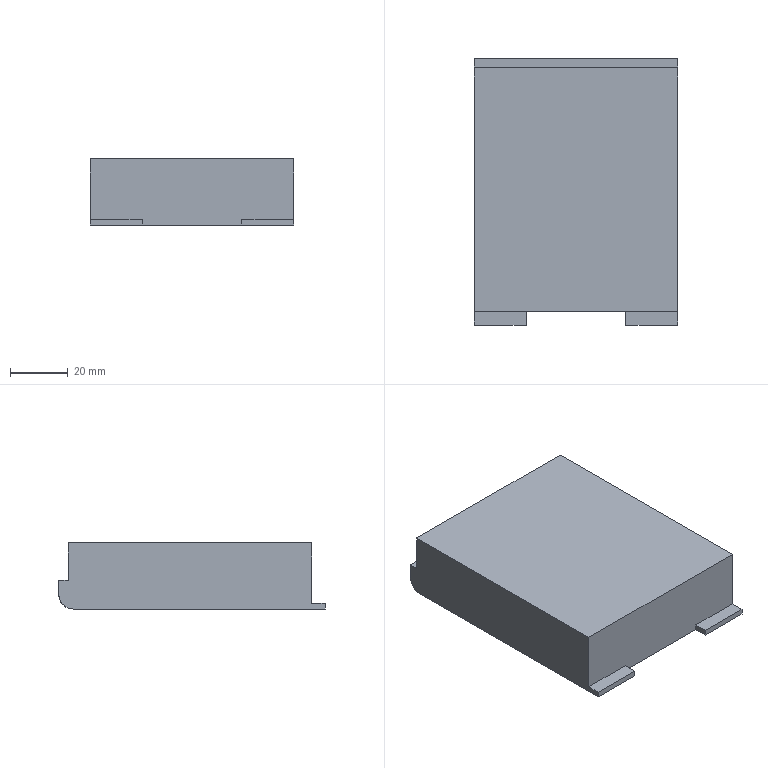Part | SolidWorks | features ICE 3, Cut 2, BossThin 1, DelFace 1, Extrusion 1, Fillet 1 | 1 solid | 35 faces | box 70.6 x 92.5 x 23 mm | volume 56360 mm3 | plane 28 | cylinder 7 | commonest cylinder face diameters 10 x4 18 x2 22 x1
STEP:
#1=CARTESIAN_POINT('',(-60.8,91.,-16.));
#2=VERTEX_POINT('',#1);
#3=CARTESIAN_POINT('',(-52.315,91.,-22.));
#4=VERTEX_POINT('',#3);
#5=CARTESIAN_POINT('',(-60.8,91.,-25.));
#6=DIRECTION('',(0.,1.,0.));
#7=DIRECTION('',(1.,0.,0.));
#8=AXIS2_PLACEMENT_3D('',#5,#6,#7);
#9=CIRCLE('',#8,9.);
#10=EDGE_CURVE('',#2,#4,#9,.T.);
#11=ORIENTED_EDGE('',*,*,#10,.F.);
#12=CARTESIAN_POINT('',(-60.8,93.,-16.));
#13=VERTEX_POINT('',#12);
#14=CARTESIAN_POINT('',(-60.8,91.,-16.));
#15=DIRECTION('',(0.,1.,0.));
#16=VECTOR('',#15,1000.);
#17=LINE('',#14,#16);
#18=EDGE_CURVE('',#2,#13,#17,.T.);
#19=ORIENTED_EDGE('',*,*,#18,.T.);
#20=CARTESIAN_POINT('',(-55.143,93.,-18.));
#21=VERTEX_POINT('',#20);
#22=CARTESIAN_POINT('',(-60.8,93.,-25.));
#23=DIRECTION('',(0.,1.,0.));
#24=DIRECTION('',(1.,0.,0.));
#25=AXIS2_PLACEMENT_3D('',#22,#23,#24);
#26=CIRCLE('',#25,9.);
#27=EDGE_CURVE('',#13,#21,#26,.T.);
#28=ORIENTED_EDGE('',*,*,#27,.T.);
#29=CARTESIAN_POINT('',(-55.143,93.,-18.));
#30=CARTESIAN_POINT('',(-54.781,93.,-18.293));
#31=CARTESIAN_POINT('',(-54.447,92.975,-18.609));
#32=CARTESIAN_POINT('',(-53.833,92.845,-19.284));
#33=CARTESIAN_POINT('',(-53.552,92.737,-19.647));
#34=CARTESIAN_POINT('',(-53.192,92.501,-20.187));
#35=CARTESIAN_POINT('',(-53.081,92.409,-20.367));
#36=CARTESIAN_POINT('',(-52.877,92.197,-20.726));
#37=CARTESIAN_POINT('',(-52.784,92.076,-20.904));
#38=CARTESIAN_POINT('',(-52.537,91.679,-21.414));
#39=CARTESIAN_POINT('',(-52.412,91.366,-21.726));
#40=CARTESIAN_POINT('',(-52.315,91.,-22.));
#41=B_SPLINE_CURVE_WITH_KNOTS('',3,(#29,#30,#31,#32,#33,#34,#35,#36,#37,#38,#39,#40),.UNSPECIFIED.,.F.,.F.,(4,2,2,2,2,4),(0.,0.00138,0.00276,0.00345,0.00414,0.00552),.UNSPECIFIED.);
#42=EDGE_CURVE('',#21,#4,#41,.T.);
#43=ORIENTED_EDGE('',*,*,#42,.T.);
#44=EDGE_LOOP('',(#11,#19,#28,#43));
#45=FACE_OUTER_BOUND('',#44,.T.);
#46=CARTESIAN_POINT('',(-60.8,91.,-25.));
#47=DIRECTION('',(0.,1.,0.));
#48=DIRECTION('',(0.,0.,1.));
#49=AXIS2_PLACEMENT_3D('',#46,#47,#48);
#50=CYLINDRICAL_SURFACE('',#49,9.);
#51=ADVANCED_FACE('',(#45),#50,.F.);
#52=CARTESIAN_POINT('',(-29.2,7.2,-23.));
#53=VERTEX_POINT('',#52);
#54=CARTESIAN_POINT('',(-29.2,7.2,-2.));
#55=VERTEX_POINT('',#54);
#56=CARTESIAN_POINT('',(-29.2,7.2,-23.));
#57=DIRECTION('',(0.,0.,1.));
#58=VECTOR('',#57,1000.);
#59=LINE('',#56,#58);
#60=EDGE_CURVE('',#53,#55,#59,.T.);
#61=ORIENTED_EDGE('',*,*,#60,.T.);
#62=CARTESIAN_POINT('',(-5.2,7.2,-2.));
#63=VERTEX_POINT('',#62);
#64=CARTESIAN_POINT('',(-48.2,7.2,-2.));
#65=DIRECTION('',(1.,0.,0.));
#66=VECTOR('',#65,1000.);
#67=LINE('',#64,#66);
#68=EDGE_CURVE('',#55,#63,#67,.T.);
#69=ORIENTED_EDGE('',*,*,#68,.T.);
#70=CARTESIAN_POINT('',(-5.2,7.2,-23.));
#71=VERTEX_POINT('',#70);
#72=CARTESIAN_POINT('',(-5.2,7.2,-2.));
#73=DIRECTION('',(0.,0.,-1.));
#74=VECTOR('',#73,1000.);
#75=LINE('',#72,#74);
#76=EDGE_CURVE('',#63,#71,#75,.T.);
#77=ORIENTED_EDGE('',*,*,#76,.T.);
#78=CARTESIAN_POINT('',(-48.2,7.2,-23.));
#79=DIRECTION('',(1.,0.,0.));
#80=VECTOR('',#79,1000.);
#81=LINE('',#78,#80);
#82=EDGE_CURVE('',#53,#71,#81,.T.);
#83=ORIENTED_EDGE('',*,*,#82,.F.);
#84=EDGE_LOOP('',(#61,#69,#77,#83));
#85=FACE_OUTER_BOUND('',#84,.T.);
#86=CARTESIAN_POINT('',(-48.2,7.2,-2.));
#87=DIRECTION('',(0.,-1.,0.));
#88=DIRECTION('',(1.,0.,0.));
#89=AXIS2_PLACEMENT_3D('',#86,#87,#88);
#90=PLANE('',#89);
#91=ADVANCED_FACE('',(#85),#90,.F.);
#92=CARTESIAN_POINT('',(-29.2,87.8,-2.));
#93=VERTEX_POINT('',#92);
#94=CARTESIAN_POINT('',(-29.2,7.2,-2.));
#95=DIRECTION('',(0.,1.,0.));
#96=VECTOR('',#95,1000.);
#97=LINE('',#94,#96);
#98=EDGE_CURVE('',#55,#93,#97,.T.);
#99=ORIENTED_EDGE('',*,*,#98,.T.);
#100=CARTESIAN_POINT('',(-5.2,87.8,-2.));
#101=VERTEX_POINT('',#100);
#102=CARTESIAN_POINT('',(-48.2,87.8,-2.));
#103=DIRECTION('',(1.,0.,0.));
#104=VECTOR('',#103,1000.);
#105=LINE('',#102,#104);
#106=EDGE_CURVE('',#93,#101,#105,.T.);
#107=ORIENTED_EDGE('',*,*,#106,.T.);
#108=CARTESIAN_POINT('',(-5.2,87.8,-2.));
#109=DIRECTION('',(0.,-1.,0.));
#110=VECTOR('',#109,1000.);
#111=LINE('',#108,#110);
#112=EDGE_CURVE('',#101,#63,#111,.T.);
#113=ORIENTED_EDGE('',*,*,#112,.T.);
#114=ORIENTED_EDGE('',*,*,#68,.F.);
#115=EDGE_LOOP('',(#99,#107,#113,#114));
#116=FACE_OUTER_BOUND('',#115,.T.);
#117=CARTESIAN_POINT('',(-48.2,87.8,-2.));
#118=DIRECTION('',(0.,0.,1.));
#119=DIRECTION('',(0.,-1.,0.));
#120=AXIS2_PLACEMENT_3D('',#117,#118,#119);
#121=PLANE('',#120);
#122=ADVANCED_FACE('',(#116),#121,.F.);
#123=CARTESIAN_POINT('',(-29.2,87.8,-15.));
#124=VERTEX_POINT('',#123);
#125=CARTESIAN_POINT('',(-29.2,87.8,-2.));
#126=DIRECTION('',(0.,0.,-1.));
#127=VECTOR('',#126,1000.);
#128=LINE('',#125,#127);
#129=EDGE_CURVE('',#93,#124,#128,.T.);
#130=ORIENTED_EDGE('',*,*,#129,.T.);
#131=CARTESIAN_POINT('',(-5.2,87.8,-15.));
#132=VERTEX_POINT('',#131);
#133=CARTESIAN_POINT('',(-48.2,87.8,-15.));
#134=DIRECTION('',(1.,0.,0.));
#135=VECTOR('',#134,1000.);
#136=LINE('',#133,#135);
#137=EDGE_CURVE('',#124,#132,#136,.T.);
#138=ORIENTED_EDGE('',*,*,#137,.T.);
#139=CARTESIAN_POINT('',(-5.2,87.8,-15.));
#140=DIRECTION('',(0.,0.,1.));
#141=VECTOR('',#140,1000.);
#142=LINE('',#139,#141);
#143=EDGE_CURVE('',#132,#101,#142,.T.);
#144=ORIENTED_EDGE('',*,*,#143,.T.);
#145=ORIENTED_EDGE('',*,*,#106,.F.);
#146=EDGE_LOOP('',(#130,#138,#144,#145));
#147=FACE_OUTER_BOUND('',#146,.T.);
#148=CARTESIAN_POINT('',(-48.2,87.8,-15.));
#149=DIRECTION('',(0.,1.,0.));
#150=DIRECTION('',(-1.,0.,0.));
#151=AXIS2_PLACEMENT_3D('',#148,#149,#150);
#152=PLANE('',#151);
#153=ADVANCED_FACE('',(#147),#152,.F.);
#154=CARTESIAN_POINT('',(-29.2,93.,-15.));
#155=VERTEX_POINT('',#154);
#156=CARTESIAN_POINT('',(-29.2,87.8,-15.));
#157=DIRECTION('',(0.,1.,0.));
#158=VECTOR('',#157,1000.);
#159=LINE('',#156,#158);
#160=EDGE_CURVE('',#124,#155,#159,.T.);
#161=ORIENTED_EDGE('',*,*,#160,.T.);
#162=CARTESIAN_POINT('',(-5.2,93.,-15.));
#163=VERTEX_POINT('',#162);
#164=CARTESIAN_POINT('',(-48.2,93.,-15.));
#165=DIRECTION('',(1.,0.,0.));
#166=VECTOR('',#165,1000.);
#167=LINE('',#164,#166);
#168=EDGE_CURVE('',#155,#163,#167,.T.);
#169=ORIENTED_EDGE('',*,*,#168,.T.);
#170=CARTESIAN_POINT('',(-5.2,93.,-15.));
#171=DIRECTION('',(0.,-1.,0.));
#172=VECTOR('',#171,1000.);
#173=LINE('',#170,#172);
#174=EDGE_CURVE('',#163,#132,#173,.T.);
#175=ORIENTED_EDGE('',*,*,#174,.T.);
#176=ORIENTED_EDGE('',*,*,#137,.F.);
#177=EDGE_LOOP('',(#161,#169,#175,#176));
#178=FACE_OUTER_BOUND('',#177,.T.);
#179=CARTESIAN_POINT('',(-48.2,93.,-15.));
#180=DIRECTION('',(0.,0.,1.));
#181=DIRECTION('',(1.,0.,0.));
#182=AXIS2_PLACEMENT_3D('',#179,#180,#181);
#183=PLANE('',#182);
#184=ADVANCED_FACE('',(#178),#183,.F.);
#185=CARTESIAN_POINT('',(-73.8,88.,-23.));
#186=VERTEX_POINT('',#185);
#187=CARTESIAN_POINT('',(-73.8,0.5,-23.));
#188=VERTEX_POINT('',#187);
#189=CARTESIAN_POINT('',(-73.8,89.8,-23.));
#190=DIRECTION('',(0.,-1.,0.));
#191=VECTOR('',#190,1000.);
#192=LINE('',#189,#191);
#193=EDGE_CURVE('',#186,#188,#192,.T.);
#194=ORIENTED_EDGE('',*,*,#193,.F.);
#195=CARTESIAN_POINT('',(-71.617,88.,-23.));
#196=VERTEX_POINT('',#195);
#197=CARTESIAN_POINT('',(0.,88.,-23.));
#198=DIRECTION('',(1.,0.,0.));
#199=VECTOR('',#198,1000.);
#200=LINE('',#197,#199);
#201=EDGE_CURVE('',#186,#196,#200,.T.);
#202=ORIENTED_EDGE('',*,*,#201,.T.);
#203=CARTESIAN_POINT('',(-71.617,7.2,-23.));
#204=VERTEX_POINT('',#203);
#205=CARTESIAN_POINT('',(-71.617,93.001,-23.));
#206=DIRECTION('',(0.,-1.,0.));
#207=VECTOR('',#206,1000.);
#208=LINE('',#205,#207);
#209=EDGE_CURVE('',#196,#204,#208,.T.);
#210=ORIENTED_EDGE('',*,*,#209,.T.);
#211=CARTESIAN_POINT('',(-49.983,7.2,-23.));
#212=VERTEX_POINT('',#211);
#213=CARTESIAN_POINT('',(-60.8,7.2,-23.));
#214=DIRECTION('',(1.,0.,0.));
#215=VECTOR('',#214,1000.);
#216=LINE('',#213,#215);
#217=EDGE_CURVE('',#204,#212,#216,.T.);
#218=ORIENTED_EDGE('',*,*,#217,.T.);
#219=CARTESIAN_POINT('',(-49.983,88.,-23.));
#220=VERTEX_POINT('',#219);
#221=CARTESIAN_POINT('',(-49.983,93.001,-23.));
#222=DIRECTION('',(0.,1.,0.));
#223=VECTOR('',#222,1000.);
#224=LINE('',#221,#223);
#225=EDGE_CURVE('',#212,#220,#224,.T.);
#226=ORIENTED_EDGE('',*,*,#225,.T.);
#227=CARTESIAN_POINT('',(-48.2,88.,-23.));
#228=VERTEX_POINT('',#227);
#229=CARTESIAN_POINT('',(0.,88.,-23.));
#230=DIRECTION('',(1.,0.,0.));
#231=VECTOR('',#230,1000.);
#232=LINE('',#229,#231);
#233=EDGE_CURVE('',#220,#228,#232,.T.);
#234=ORIENTED_EDGE('',*,*,#233,.T.);
#235=CARTESIAN_POINT('',(-48.2,7.2,-23.));
#236=VERTEX_POINT('',#235);
#237=CARTESIAN_POINT('',(-48.2,7.2,-23.));
#238=DIRECTION('',(0.,1.,0.));
#239=VECTOR('',#238,1000.);
#240=LINE('',#237,#239);
#241=EDGE_CURVE('',#236,#228,#240,.T.);
#242=ORIENTED_EDGE('',*,*,#241,.F.);
#243=CARTESIAN_POINT('',(-31.2,7.2,-23.));
#244=VERTEX_POINT('',#243);
#245=CARTESIAN_POINT('',(-48.2,7.2,-23.));
#246=DIRECTION('',(1.,0.,0.));
#247=VECTOR('',#246,1000.);
#248=LINE('',#245,#247);
#249=EDGE_CURVE('',#236,#244,#248,.T.);
#250=ORIENTED_EDGE('',*,*,#249,.T.);
#251=CARTESIAN_POINT('',(-31.2,88.,-23.));
#252=VERTEX_POINT('',#251);
#253=CARTESIAN_POINT('',(-31.2,93.,-23.));
#254=DIRECTION('',(0.,-1.,0.));
#255=VECTOR('',#254,1000.);
#256=LINE('',#253,#255);
#257=EDGE_CURVE('',#252,#244,#256,.T.);
#258=ORIENTED_EDGE('',*,*,#257,.F.);
#259=CARTESIAN_POINT('',(-29.2,88.,-23.));
#260=VERTEX_POINT('',#259);
#261=CARTESIAN_POINT('',(0.,88.,-23.));
#262=DIRECTION('',(1.,0.,0.));
#263=VECTOR('',#262,1000.);
#264=LINE('',#261,#263);
#265=EDGE_CURVE('',#252,#260,#264,.T.);
#266=ORIENTED_EDGE('',*,*,#265,.T.);
#267=CARTESIAN_POINT('',(-29.2,93.,-23.));
#268=DIRECTION('',(0.,-1.,0.));
#269=VECTOR('',#268,1000.);
#270=LINE('',#267,#269);
#271=EDGE_CURVE('',#260,#53,#270,.T.);
#272=ORIENTED_EDGE('',*,*,#271,.T.);
#273=ORIENTED_EDGE('',*,*,#82,.T.);
#274=CARTESIAN_POINT('',(-5.2,88.,-23.));
#275=VERTEX_POINT('',#274);
#276=CARTESIAN_POINT('',(-5.2,7.2,-23.));
#277=DIRECTION('',(0.,1.,0.));
#278=VECTOR('',#277,1000.);
#279=LINE('',#276,#278);
#280=EDGE_CURVE('',#71,#275,#279,.T.);
#281=ORIENTED_EDGE('',*,*,#280,.T.);
#282=CARTESIAN_POINT('',(-3.2,88.,-23.));
#283=VERTEX_POINT('',#282);
#284=CARTESIAN_POINT('',(0.,88.,-23.));
#285=DIRECTION('',(1.,0.,0.));
#286=VECTOR('',#285,1000.);
#287=LINE('',#284,#286);
#288=EDGE_CURVE('',#275,#283,#287,.T.);
#289=ORIENTED_EDGE('',*,*,#288,.T.);
#290=CARTESIAN_POINT('',(-3.2,0.5,-23.));
#291=VERTEX_POINT('',#290);
#292=CARTESIAN_POINT('',(-3.2,89.8,-23.));
#293=DIRECTION('',(0.,1.,0.));
#294=VECTOR('',#293,1000.);
#295=LINE('',#292,#294);
#296=EDGE_CURVE('',#291,#283,#295,.T.);
#297=ORIENTED_EDGE('',*,*,#296,.F.);
#298=CARTESIAN_POINT('',(-21.2,0.5,-23.));
#299=VERTEX_POINT('',#298);
#300=CARTESIAN_POINT('',(-3.2,0.5,-23.));
#301=DIRECTION('',(-1.,0.,0.));
#302=VECTOR('',#301,1000.);
#303=LINE('',#300,#302);
#304=EDGE_CURVE('',#291,#299,#303,.T.);
#305=ORIENTED_EDGE('',*,*,#304,.T.);
#306=CARTESIAN_POINT('',(-21.2,5.2,-23.));
#307=VERTEX_POINT('',#306);
#308=CARTESIAN_POINT('',(-21.2,5.2,-23.));
#309=DIRECTION('',(0.,1.,0.));
#310=VECTOR('',#309,1000.);
#311=LINE('',#308,#310);
#312=EDGE_CURVE('',#299,#307,#311,.T.);
#313=ORIENTED_EDGE('',*,*,#312,.T.);
#314=CARTESIAN_POINT('',(-55.8,5.2,-23.));
#315=VERTEX_POINT('',#314);
#316=CARTESIAN_POINT('',(-73.8,5.2,-23.));
#317=DIRECTION('',(1.,0.,0.));
#318=VECTOR('',#317,1000.);
#319=LINE('',#316,#318);
#320=EDGE_CURVE('',#315,#307,#319,.T.);
#321=ORIENTED_EDGE('',*,*,#320,.F.);
#322=CARTESIAN_POINT('',(-55.8,0.5,-23.));
#323=VERTEX_POINT('',#322);
#324=CARTESIAN_POINT('',(-55.8,5.2,-23.));
#325=DIRECTION('',(0.,-1.,0.));
#326=VECTOR('',#325,1000.);
#327=LINE('',#324,#326);
#328=EDGE_CURVE('',#315,#323,#327,.T.);
#329=ORIENTED_EDGE('',*,*,#328,.T.);
#330=CARTESIAN_POINT('',(-73.8,0.5,-23.));
#331=DIRECTION('',(-1.,0.,0.));
#332=VECTOR('',#331,1000.);
#333=LINE('',#330,#332);
#334=EDGE_CURVE('',#323,#188,#333,.T.);
#335=ORIENTED_EDGE('',*,*,#334,.T.);
#336=EDGE_LOOP('',(#194,#202,#210,#218,#226,#234,#242,#250,#258,#266,#272,#273,#281,#289,#297,#305,#313,#321,#329,#335));
#337=FACE_OUTER_BOUND('',#336,.T.);
#338=CARTESIAN_POINT('',(0.,0.,-23.));
#339=DIRECTION('',(0.,0.,-1.));
#340=DIRECTION('',(0.,-1.,0.));
#341=AXIS2_PLACEMENT_3D('',#338,#339,#340);
#342=PLANE('',#341);
#343=ADVANCED_FACE('',(#337),#342,.T.);
#344=CARTESIAN_POINT('',(-66.457,93.,-18.));
#345=VERTEX_POINT('',#344);
#346=CARTESIAN_POINT('',(-60.8,93.,-25.));
#347=DIRECTION('',(0.,1.,0.));
#348=DIRECTION('',(1.,0.,0.));
#349=AXIS2_PLACEMENT_3D('',#346,#347,#348);
#350=CIRCLE('',#349,9.);
#351=EDGE_CURVE('',#345,#13,#350,.T.);
#352=ORIENTED_EDGE('',*,*,#351,.F.);
#353=CARTESIAN_POINT('',(-73.8,93.,-18.));
#354=VERTEX_POINT('',#353);
#355=CARTESIAN_POINT('',(-3.2,93.,-18.));
#356=DIRECTION('',(-1.,0.,0.));
#357=VECTOR('',#356,1000.);
#358=LINE('',#355,#357);
#359=EDGE_CURVE('',#345,#354,#358,.T.);
#360=ORIENTED_EDGE('',*,*,#359,.T.);
#361=CARTESIAN_POINT('',(-73.8,93.,-13.));
#362=VERTEX_POINT('',#361);
#363=CARTESIAN_POINT('',(-73.8,93.,57.672));
#364=DIRECTION('',(0.,0.,-1.));
#365=VECTOR('',#364,1000.);
#366=LINE('',#363,#365);
#367=EDGE_CURVE('',#362,#354,#366,.T.);
#368=ORIENTED_EDGE('',*,*,#367,.F.);
#369=CARTESIAN_POINT('',(-3.2,93.,-13.));
#370=VERTEX_POINT('',#369);
#371=CARTESIAN_POINT('',(-3.2,93.,-13.));
#372=DIRECTION('',(1.,0.,0.));
#373=VECTOR('',#372,1000.);
#374=LINE('',#371,#373);
#375=EDGE_CURVE('',#362,#370,#374,.T.);
#376=ORIENTED_EDGE('',*,*,#375,.T.);
#377=CARTESIAN_POINT('',(-3.2,93.,-18.));
#378=VERTEX_POINT('',#377);
#379=CARTESIAN_POINT('',(-3.2,93.,57.672));
#380=DIRECTION('',(0.,0.,-1.));
#381=VECTOR('',#380,1000.);
#382=LINE('',#379,#381);
#383=EDGE_CURVE('',#370,#378,#382,.T.);
#384=ORIENTED_EDGE('',*,*,#383,.T.);
#385=CARTESIAN_POINT('',(-5.2,93.,-18.));
#386=VERTEX_POINT('',#385);
#387=CARTESIAN_POINT('',(-3.2,93.,-18.));
#388=DIRECTION('',(-1.,0.,0.));
#389=VECTOR('',#388,1000.);
#390=LINE('',#387,#389);
#391=EDGE_CURVE('',#378,#386,#390,.T.);
#392=ORIENTED_EDGE('',*,*,#391,.T.);
#393=CARTESIAN_POINT('',(-5.2,93.,-23.));
#394=DIRECTION('',(0.,0.,1.));
#395=VECTOR('',#394,1000.);
#396=LINE('',#393,#395);
#397=EDGE_CURVE('',#386,#163,#396,.T.);
#398=ORIENTED_EDGE('',*,*,#397,.T.);
#399=ORIENTED_EDGE('',*,*,#168,.F.);
#400=CARTESIAN_POINT('',(-29.2,93.,-18.));
#401=VERTEX_POINT('',#400);
#402=CARTESIAN_POINT('',(-29.2,93.,-15.));
#403=DIRECTION('',(0.,0.,-1.));
#404=VECTOR('',#403,1000.);
#405=LINE('',#402,#404);
#406=EDGE_CURVE('',#155,#401,#405,.T.);
#407=ORIENTED_EDGE('',*,*,#406,.T.);
#408=CARTESIAN_POINT('',(-31.2,93.,-18.));
#409=VERTEX_POINT('',#408);
#410=CARTESIAN_POINT('',(-3.2,93.,-18.));
#411=DIRECTION('',(-1.,0.,0.));
#412=VECTOR('',#411,1000.);
#413=LINE('',#410,#412);
#414=EDGE_CURVE('',#401,#409,#413,.T.);
#415=ORIENTED_EDGE('',*,*,#414,.T.);
#416=CARTESIAN_POINT('',(-31.2,93.,-15.));
#417=VERTEX_POINT('',#416);
#418=CARTESIAN_POINT('',(-31.2,93.,-15.));
#419=DIRECTION('',(0.,0.,-1.));
#420=VECTOR('',#419,1000.);
#421=LINE('',#418,#420);
#422=EDGE_CURVE('',#417,#409,#421,.T.);
#423=ORIENTED_EDGE('',*,*,#422,.F.);
#424=CARTESIAN_POINT('',(-48.2,93.,-15.));
#425=VERTEX_POINT('',#424);
#426=CARTESIAN_POINT('',(-48.2,93.,-15.));
#427=DIRECTION('',(1.,0.,0.));
#428=VECTOR('',#427,1000.);
#429=LINE('',#426,#428);
#430=EDGE_CURVE('',#425,#417,#429,.T.);
#431=ORIENTED_EDGE('',*,*,#430,.F.);
#432=CARTESIAN_POINT('',(-48.2,93.,-18.));
#433=VERTEX_POINT('',#432);
#434=CARTESIAN_POINT('',(-48.2,93.,-23.));
#435=DIRECTION('',(0.,0.,1.));
#436=VECTOR('',#435,1000.);
#437=LINE('',#434,#436);
#438=EDGE_CURVE('',#433,#425,#437,.T.);
#439=ORIENTED_EDGE('',*,*,#438,.F.);
#440=CARTESIAN_POINT('',(-3.2,93.,-18.));
#441=DIRECTION('',(-1.,0.,0.));
#442=VECTOR('',#441,1000.);
#443=LINE('',#440,#442);
#444=EDGE_CURVE('',#433,#21,#443,.T.);
#445=ORIENTED_EDGE('',*,*,#444,.T.);
#446=ORIENTED_EDGE('',*,*,#27,.F.);
#447=EDGE_LOOP('',(#352,#360,#368,#376,#384,#392,#398,#399,#407,#415,#423,#431,#439,#445,#446));
#448=FACE_OUTER_BOUND('',#447,.T.);
#449=CARTESIAN_POINT('',(-3.2,93.,57.672));
#450=DIRECTION('',(0.,1.,0.));
#451=DIRECTION('',(0.,0.,1.));
#452=AXIS2_PLACEMENT_3D('',#449,#450,#451);
#453=PLANE('',#452);
#454=ADVANCED_FACE('',(#448),#453,.T.);
#455=ORIENTED_EDGE('',*,*,#209,.F.);
#456=CARTESIAN_POINT('',(-71.383,91.,-22.));
#457=VERTEX_POINT('',#456);
#458=CARTESIAN_POINT('',(-71.617,88.,-23.));
#459=CARTESIAN_POINT('',(-71.617,88.543,-23.));
#460=CARTESIAN_POINT('',(-71.602,89.072,-22.914));
#461=CARTESIAN_POINT('',(-71.53,90.099,-22.57));
#462=CARTESIAN_POINT('',(-71.474,90.571,-22.321));
#463=CARTESIAN_POINT('',(-71.383,91.,-22.));
#464=B_SPLINE_CURVE_WITH_KNOTS('',3,(#458,#459,#460,#461,#462,#463),.UNSPECIFIED.,.F.,.F.,(4,2,4),(0.,0.001607,0.003214),.UNSPECIFIED.);
#465=EDGE_CURVE('',#196,#457,#464,.T.);
#466=ORIENTED_EDGE('',*,*,#465,.T.);
#467=CARTESIAN_POINT('',(-50.217,91.,-22.));
#468=VERTEX_POINT('',#467);
#469=CARTESIAN_POINT('',(-60.8,91.,-25.));
#470=DIRECTION('',(0.,1.,0.));
#471=DIRECTION('',(0.,0.,1.));
#472=AXIS2_PLACEMENT_3D('',#469,#470,#471);
#473=CIRCLE('',#472,11.);
#474=EDGE_CURVE('',#457,#468,#473,.T.);
#475=ORIENTED_EDGE('',*,*,#474,.T.);
#476=CARTESIAN_POINT('',(-50.217,91.,-22.));
#477=CARTESIAN_POINT('',(-50.126,90.571,-22.321));
#478=CARTESIAN_POINT('',(-50.07,90.1,-22.57));
#479=CARTESIAN_POINT('',(-49.998,89.073,-22.913));
#480=CARTESIAN_POINT('',(-49.983,88.543,-23.));
#481=CARTESIAN_POINT('',(-49.983,88.,-23.));
#482=B_SPLINE_CURVE_WITH_KNOTS('',3,(#476,#477,#478,#479,#480,#481),.UNSPECIFIED.,.F.,.F.,(4,2,4),(0.,0.001607,0.003213),.UNSPECIFIED.);
#483=EDGE_CURVE('',#468,#220,#482,.T.);
#484=ORIENTED_EDGE('',*,*,#483,.T.);
#485=ORIENTED_EDGE('',*,*,#225,.F.);
#486=CARTESIAN_POINT('',(-60.8,7.2,-25.));
#487=DIRECTION('',(0.,-1.,0.));
#488=DIRECTION('',(0.,0.,-1.));
#489=AXIS2_PLACEMENT_3D('',#486,#487,#488);
#490=CIRCLE('',#489,11.);
#491=EDGE_CURVE('',#212,#204,#490,.T.);
#492=ORIENTED_EDGE('',*,*,#491,.T.);
#493=EDGE_LOOP('',(#455,#466,#475,#484,#485,#492));
#494=FACE_OUTER_BOUND('',#493,.T.);
#495=CARTESIAN_POINT('',(-60.8,93.001,-25.));
#496=DIRECTION('',(0.,-1.,0.));
#497=DIRECTION('',(0.,0.,-1.));
#498=AXIS2_PLACEMENT_3D('',#495,#496,#497);
#499=CYLINDRICAL_SURFACE('',#498,11.);
#500=ADVANCED_FACE('',(#494),#499,.F.);
#501=CARTESIAN_POINT('',(-3.2,89.8,-13.));
#502=VERTEX_POINT('',#501);
#503=CARTESIAN_POINT('',(-3.2,89.8,0.));
#504=VERTEX_POINT('',#503);
#505=CARTESIAN_POINT('',(-3.2,89.8,-133.189));
#506=DIRECTION('',(0.,0.,1.));
#507=VECTOR('',#506,1000.);
#508=LINE('',#505,#507);
#509=EDGE_CURVE('',#502,#504,#508,.T.);
#510=ORIENTED_EDGE('',*,*,#509,.F.);
#511=CARTESIAN_POINT('',(-73.8,89.8,-13.));
#512=VERTEX_POINT('',#511);
#513=CARTESIAN_POINT('',(-3.2,89.8,-13.));
#514=DIRECTION('',(-1.,0.,0.));
#515=VECTOR('',#514,1000.);
#516=LINE('',#513,#515);
#517=EDGE_CURVE('',#502,#512,#516,.T.);
#518=ORIENTED_EDGE('',*,*,#517,.T.);
#519=CARTESIAN_POINT('',(-73.8,89.8,0.));
#520=VERTEX_POINT('',#519);
#521=CARTESIAN_POINT('',(-73.8,89.8,-133.189));
#522=DIRECTION('',(0.,0.,1.));
#523=VECTOR('',#522,1000.);
#524=LINE('',#521,#523);
#525=EDGE_CURVE('',#512,#520,#524,.T.);
#526=ORIENTED_EDGE('',*,*,#525,.T.);
#527=CARTESIAN_POINT('',(-73.8,89.8,0.));
#528=DIRECTION('',(-1.,0.,0.));
#529=VECTOR('',#528,1000.);
#530=LINE('',#527,#529);
#531=EDGE_CURVE('',#504,#520,#530,.T.);
#532=ORIENTED_EDGE('',*,*,#531,.F.);
#533=EDGE_LOOP('',(#510,#518,#526,#532));
#534=FACE_OUTER_BOUND('',#533,.T.);
#535=CARTESIAN_POINT('',(-73.8,89.8,-133.189));
#536=DIRECTION('',(0.,1.,0.));
#537=DIRECTION('',(0.,0.,1.));
#538=AXIS2_PLACEMENT_3D('',#535,#536,#537);
#539=PLANE('',#538);
#540=ADVANCED_FACE('',(#534),#539,.T.);
#541=CARTESIAN_POINT('',(-73.8,5.2,0.));
#542=VERTEX_POINT('',#541);
#543=CARTESIAN_POINT('',(-73.8,89.8,0.));
#544=DIRECTION('',(0.,-1.,0.));
#545=VECTOR('',#544,1000.);
#546=LINE('',#543,#545);
#547=EDGE_CURVE('',#520,#542,#546,.T.);
#548=ORIENTED_EDGE('',*,*,#547,.T.);
#549=CARTESIAN_POINT('',(-3.2,5.2,0.));
#550=VERTEX_POINT('',#549);
#551=CARTESIAN_POINT('',(-73.8,5.2,0.));
#552=DIRECTION('',(1.,0.,0.));
#553=VECTOR('',#552,1000.);
#554=LINE('',#551,#553);
#555=EDGE_CURVE('',#542,#550,#554,.T.);
#556=ORIENTED_EDGE('',*,*,#555,.T.);
#557=CARTESIAN_POINT('',(-3.2,89.8,0.));
#558=DIRECTION('',(0.,1.,0.));
#559=VECTOR('',#558,1000.);
#560=LINE('',#557,#559);
#561=EDGE_CURVE('',#550,#504,#560,.T.);
#562=ORIENTED_EDGE('',*,*,#561,.T.);
#563=ORIENTED_EDGE('',*,*,#531,.T.);
#564=EDGE_LOOP('',(#548,#556,#562,#563));
#565=FACE_OUTER_BOUND('',#564,.T.);
#566=CARTESIAN_POINT('',(0.,0.,0.));
#567=DIRECTION('',(0.,0.,1.));
#568=DIRECTION('',(1.,0.,0.));
#569=AXIS2_PLACEMENT_3D('',#566,#567,#568);
#570=PLANE('',#569);
#571=ADVANCED_FACE('',(#565),#570,.T.);
#572=CARTESIAN_POINT('',(-55.8,5.2,-21.));
#573=VERTEX_POINT('',#572);
#574=CARTESIAN_POINT('',(-55.8,5.2,-21.));
#575=DIRECTION('',(0.,0.,-1.));
#576=VECTOR('',#575,1000.);
#577=LINE('',#574,#576);
#578=EDGE_CURVE('',#573,#315,#577,.T.);
#579=ORIENTED_EDGE('',*,*,#578,.T.);
#580=ORIENTED_EDGE('',*,*,#320,.T.);
#581=CARTESIAN_POINT('',(-21.2,5.2,-21.));
#582=VERTEX_POINT('',#581);
#583=CARTESIAN_POINT('',(-21.2,5.2,-21.));
#584=DIRECTION('',(0.,0.,-1.));
#585=VECTOR('',#584,1000.);
#586=LINE('',#583,#585);
#587=EDGE_CURVE('',#582,#307,#586,.T.);
#588=ORIENTED_EDGE('',*,*,#587,.F.);
#589=CARTESIAN_POINT('',(-3.2,5.2,-21.));
#590=VERTEX_POINT('',#589);
#591=CARTESIAN_POINT('',(-3.2,5.2,-21.));
#592=DIRECTION('',(1.,0.,0.));
#593=VECTOR('',#592,1000.);
#594=LINE('',#591,#593);
#595=EDGE_CURVE('',#582,#590,#594,.T.);
#596=ORIENTED_EDGE('',*,*,#595,.T.);
#597=CARTESIAN_POINT('',(-3.2,5.2,-133.189));
#598=DIRECTION('',(0.,0.,1.));
#599=VECTOR('',#598,1000.);
#600=LINE('',#597,#599);
#601=EDGE_CURVE('',#590,#550,#600,.T.);
#602=ORIENTED_EDGE('',*,*,#601,.T.);
#603=ORIENTED_EDGE('',*,*,#555,.F.);
#604=CARTESIAN_POINT('',(-73.8,5.2,-21.));
#605=VERTEX_POINT('',#604);
#606=CARTESIAN_POINT('',(-73.8,5.2,-133.189));
#607=DIRECTION('',(0.,0.,1.));
#608=VECTOR('',#607,1000.);
#609=LINE('',#606,#608);
#610=EDGE_CURVE('',#605,#542,#609,.T.);
#611=ORIENTED_EDGE('',*,*,#610,.F.);
#612=CARTESIAN_POINT('',(-73.8,5.2,-21.));
#613=DIRECTION('',(1.,0.,0.));
#614=VECTOR('',#613,1000.);
#615=LINE('',#612,#614);
#616=EDGE_CURVE('',#605,#573,#615,.T.);
#617=ORIENTED_EDGE('',*,*,#616,.T.);
#618=EDGE_LOOP('',(#579,#580,#588,#596,#602,#603,#611,#617));
#619=FACE_OUTER_BOUND('',#618,.T.);
#620=CARTESIAN_POINT('',(-73.8,5.2,-133.189));
#621=DIRECTION('',(0.,-1.,0.));
#622=DIRECTION('',(0.,0.,-1.));
#623=AXIS2_PLACEMENT_3D('',#620,#621,#622);
#624=PLANE('',#623);
#625=ADVANCED_FACE('',(#619),#624,.T.);
#626=ORIENTED_EDGE('',*,*,#296,.T.);
#627=CARTESIAN_POINT('',(-3.2,88.,-18.));
#628=DIRECTION('',(1.,0.,0.));
#629=DIRECTION('',(0.,1.,0.));
#630=AXIS2_PLACEMENT_3D('',#627,#628,#629);
#631=CIRCLE('',#630,5.);
#632=EDGE_CURVE('',#283,#378,#631,.T.);
#633=ORIENTED_EDGE('',*,*,#632,.T.);
#634=ORIENTED_EDGE('',*,*,#383,.F.);
#635=CARTESIAN_POINT('',(-3.2,89.8,-13.));
#636=DIRECTION('',(0.,-1.,0.));
#637=VECTOR('',#636,1000.);
#638=LINE('',#635,#637);
#639=EDGE_CURVE('',#370,#502,#638,.T.);
#640=ORIENTED_EDGE('',*,*,#639,.T.);
#641=ORIENTED_EDGE('',*,*,#509,.T.);
#642=ORIENTED_EDGE('',*,*,#561,.F.);
#643=ORIENTED_EDGE('',*,*,#601,.F.);
#644=CARTESIAN_POINT('',(-3.2,0.5,-21.));
#645=VERTEX_POINT('',#644);
#646=CARTESIAN_POINT('',(-3.2,5.2,-21.));
#647=DIRECTION('',(0.,-1.,0.));
#648=VECTOR('',#647,1000.);
#649=LINE('',#646,#648);
#650=EDGE_CURVE('',#590,#645,#649,.T.);
#651=ORIENTED_EDGE('',*,*,#650,.T.);
#652=CARTESIAN_POINT('',(-3.2,0.5,-21.));
#653=DIRECTION('',(0.,0.,-1.));
#654=VECTOR('',#653,1000.);
#655=LINE('',#652,#654);
#656=EDGE_CURVE('',#645,#291,#655,.T.);
#657=ORIENTED_EDGE('',*,*,#656,.T.);
#658=EDGE_LOOP('',(#626,#633,#634,#640,#641,#642,#643,#651,#657));
#659=FACE_OUTER_BOUND('',#658,.T.);
#660=CARTESIAN_POINT('',(-3.2,89.8,-133.189));
#661=DIRECTION('',(1.,0.,0.));
#662=DIRECTION('',(0.,1.,0.));
#663=AXIS2_PLACEMENT_3D('',#660,#661,#662);
#664=PLANE('',#663);
#665=ADVANCED_FACE('',(#659),#664,.T.);
#666=ORIENTED_EDGE('',*,*,#367,.T.);
#667=CARTESIAN_POINT('',(-73.8,88.,-18.));
#668=DIRECTION('',(-1.,0.,0.));
#669=DIRECTION('',(0.,-1.,0.));
#670=AXIS2_PLACEMENT_3D('',#667,#668,#669);
#671=CIRCLE('',#670,5.);
#672=EDGE_CURVE('',#354,#186,#671,.T.);
#673=ORIENTED_EDGE('',*,*,#672,.T.);
#674=ORIENTED_EDGE('',*,*,#193,.T.);
#675=CARTESIAN_POINT('',(-73.8,0.5,-21.));
#676=VERTEX_POINT('',#675);
#677=CARTESIAN_POINT('',(-73.8,0.5,-21.));
#678=DIRECTION('',(0.,0.,-1.));
#679=VECTOR('',#678,1000.);
#680=LINE('',#677,#679);
#681=EDGE_CURVE('',#676,#188,#680,.T.);
#682=ORIENTED_EDGE('',*,*,#681,.F.);
#683=CARTESIAN_POINT('',(-73.8,5.2,-21.));
#684=DIRECTION('',(0.,1.,0.));
#685=VECTOR('',#684,1000.);
#686=LINE('',#683,#685);
#687=EDGE_CURVE('',#676,#605,#686,.T.);
#688=ORIENTED_EDGE('',*,*,#687,.T.);
#689=ORIENTED_EDGE('',*,*,#610,.T.);
#690=ORIENTED_EDGE('',*,*,#547,.F.);
#691=ORIENTED_EDGE('',*,*,#525,.F.);
#692=CARTESIAN_POINT('',(-73.8,89.8,-13.));
#693=DIRECTION('',(0.,1.,0.));
#694=VECTOR('',#693,1000.);
#695=LINE('',#692,#694);
#696=EDGE_CURVE('',#512,#362,#695,.T.);
#697=ORIENTED_EDGE('',*,*,#696,.T.);
#698=EDGE_LOOP('',(#666,#673,#674,#682,#688,#689,#690,#691,#697));
#699=FACE_OUTER_BOUND('',#698,.T.);
#700=CARTESIAN_POINT('',(-73.8,89.8,-133.189));
#701=DIRECTION('',(-1.,0.,0.));
#702=DIRECTION('',(0.,-1.,0.));
#703=AXIS2_PLACEMENT_3D('',#700,#701,#702);
#704=PLANE('',#703);
#705=ADVANCED_FACE('',(#699),#704,.T.);
#706=ORIENTED_EDGE('',*,*,#312,.F.);
#707=CARTESIAN_POINT('',(-21.2,0.5,-21.));
#708=VERTEX_POINT('',#707);
#709=CARTESIAN_POINT('',(-21.2,0.5,-21.));
#710=DIRECTION('',(0.,0.,-1.));
#711=VECTOR('',#710,1000.);
#712=LINE('',#709,#711);
#713=EDGE_CURVE('',#708,#299,#712,.T.);
#714=ORIENTED_EDGE('',*,*,#713,.F.);
#715=CARTESIAN_POINT('',(-21.2,5.2,-21.));
#716=DIRECTION('',(0.,1.,0.));
#717=VECTOR('',#716,1000.);
#718=LINE('',#715,#717);
#719=EDGE_CURVE('',#708,#582,#718,.T.);
#720=ORIENTED_EDGE('',*,*,#719,.T.);
#721=ORIENTED_EDGE('',*,*,#587,.T.);
#722=EDGE_LOOP('',(#706,#714,#720,#721));
#723=FACE_OUTER_BOUND('',#722,.T.);
#724=CARTESIAN_POINT('',(-21.2,5.2,-21.));
#725=DIRECTION('',(-1.,0.,0.));
#726=DIRECTION('',(0.,0.,1.));
#727=AXIS2_PLACEMENT_3D('',#724,#725,#726);
#728=PLANE('',#727);
#729=ADVANCED_FACE('',(#723),#728,.T.);
#730=ORIENTED_EDGE('',*,*,#304,.F.);
#731=ORIENTED_EDGE('',*,*,#656,.F.);
#732=CARTESIAN_POINT('',(-3.2,0.5,-21.));
#733=DIRECTION('',(-1.,0.,0.));
#734=VECTOR('',#733,1000.);
#735=LINE('',#732,#734);
#736=EDGE_CURVE('',#645,#708,#735,.T.);
#737=ORIENTED_EDGE('',*,*,#736,.T.);
#738=ORIENTED_EDGE('',*,*,#713,.T.);
#739=EDGE_LOOP('',(#730,#731,#737,#738));
#740=FACE_OUTER_BOUND('',#739,.T.);
#741=CARTESIAN_POINT('',(-3.2,0.5,-21.));
#742=DIRECTION('',(0.,-1.,0.));
#743=DIRECTION('',(0.,0.,-1.));
#744=AXIS2_PLACEMENT_3D('',#741,#742,#743);
#745=PLANE('',#744);
#746=ADVANCED_FACE('',(#740),#745,.T.);
#747=ORIENTED_EDGE('',*,*,#650,.F.);
#748=ORIENTED_EDGE('',*,*,#595,.F.);
#749=ORIENTED_EDGE('',*,*,#719,.F.);
#750=ORIENTED_EDGE('',*,*,#736,.F.);
#751=EDGE_LOOP('',(#747,#748,#749,#750));
#752=FACE_OUTER_BOUND('',#751,.T.);
#753=CARTESIAN_POINT('',(0.,0.,-21.));
#754=DIRECTION('',(0.,0.,-1.));
#755=DIRECTION('',(-1.,0.,0.));
#756=AXIS2_PLACEMENT_3D('',#753,#754,#755);
#757=PLANE('',#756);
#758=ADVANCED_FACE('',(#752),#757,.F.);
#759=ORIENTED_EDGE('',*,*,#334,.F.);
#760=CARTESIAN_POINT('',(-55.8,0.5,-21.));
#761=VERTEX_POINT('',#760);
#762=CARTESIAN_POINT('',(-55.8,0.5,-21.));
#763=DIRECTION('',(0.,0.,-1.));
#764=VECTOR('',#763,1000.);
#765=LINE('',#762,#764);
#766=EDGE_CURVE('',#761,#323,#765,.T.);
#767=ORIENTED_EDGE('',*,*,#766,.F.);
#768=CARTESIAN_POINT('',(-73.8,0.5,-21.));
#769=DIRECTION('',(-1.,0.,0.));
#770=VECTOR('',#769,1000.);
#771=LINE('',#768,#770);
#772=EDGE_CURVE('',#761,#676,#771,.T.);
#773=ORIENTED_EDGE('',*,*,#772,.T.);
#774=ORIENTED_EDGE('',*,*,#681,.T.);
#775=EDGE_LOOP('',(#759,#767,#773,#774));
#776=FACE_OUTER_BOUND('',#775,.T.);
#777=CARTESIAN_POINT('',(-73.8,0.5,-21.));
#778=DIRECTION('',(0.,-1.,0.));
#779=DIRECTION('',(0.,0.,-1.));
#780=AXIS2_PLACEMENT_3D('',#777,#778,#779);
#781=PLANE('',#780);
#782=ADVANCED_FACE('',(#776),#781,.T.);
#783=ORIENTED_EDGE('',*,*,#328,.F.);
#784=ORIENTED_EDGE('',*,*,#578,.F.);
#785=CARTESIAN_POINT('',(-55.8,5.2,-21.));
#786=DIRECTION('',(0.,-1.,0.));
#787=VECTOR('',#786,1000.);
#788=LINE('',#785,#787);
#789=EDGE_CURVE('',#573,#761,#788,.T.);
#790=ORIENTED_EDGE('',*,*,#789,.T.);
#791=ORIENTED_EDGE('',*,*,#766,.T.);
#792=EDGE_LOOP('',(#783,#784,#790,#791));
#793=FACE_OUTER_BOUND('',#792,.T.);
#794=CARTESIAN_POINT('',(-55.8,5.2,-21.));
#795=DIRECTION('',(1.,0.,0.));
#796=DIRECTION('',(0.,0.,-1.));
#797=AXIS2_PLACEMENT_3D('',#794,#795,#796);
#798=PLANE('',#797);
#799=ADVANCED_FACE('',(#793),#798,.T.);
#800=ORIENTED_EDGE('',*,*,#616,.F.);
#801=ORIENTED_EDGE('',*,*,#687,.F.);
#802=ORIENTED_EDGE('',*,*,#772,.F.);
#803=ORIENTED_EDGE('',*,*,#789,.F.);
#804=EDGE_LOOP('',(#800,#801,#802,#803));
#805=FACE_OUTER_BOUND('',#804,.T.);
#806=CARTESIAN_POINT('',(0.,0.,-21.));
#807=DIRECTION('',(0.,0.,-1.));
#808=DIRECTION('',(-1.,0.,0.));
#809=AXIS2_PLACEMENT_3D('',#806,#807,#808);
#810=PLANE('',#809);
#811=ADVANCED_FACE('',(#805),#810,.F.);
#812=ORIENTED_EDGE('',*,*,#639,.F.);
#813=ORIENTED_EDGE('',*,*,#375,.F.);
#814=ORIENTED_EDGE('',*,*,#696,.F.);
#815=ORIENTED_EDGE('',*,*,#517,.F.);
#816=EDGE_LOOP('',(#812,#813,#814,#815));
#817=FACE_OUTER_BOUND('',#816,.T.);
#818=CARTESIAN_POINT('',(0.,0.,-13.));
#819=DIRECTION('',(0.,0.,1.));
#820=DIRECTION('',(-1.,0.,0.));
#821=AXIS2_PLACEMENT_3D('',#818,#819,#820);
#822=PLANE('',#821);
#823=ADVANCED_FACE('',(#817),#822,.T.);
#824=ORIENTED_EDGE('',*,*,#491,.F.);
#825=ORIENTED_EDGE('',*,*,#217,.F.);
#826=EDGE_LOOP('',(#824,#825));
#827=FACE_OUTER_BOUND('',#826,.T.);
#828=CARTESIAN_POINT('',(-60.8,7.2,-25.));
#829=DIRECTION('',(0.,-1.,0.));
#830=DIRECTION('',(0.,0.,-1.));
#831=AXIS2_PLACEMENT_3D('',#828,#829,#830);
#832=PLANE('',#831);
#833=ADVANCED_FACE('',(#827),#832,.F.);
#834=ORIENTED_EDGE('',*,*,#18,.F.);
#835=CARTESIAN_POINT('',(-69.285,91.,-22.));
#836=VERTEX_POINT('',#835);
#837=CARTESIAN_POINT('',(-60.8,91.,-25.));
#838=DIRECTION('',(0.,1.,0.));
#839=DIRECTION('',(1.,0.,0.));
#840=AXIS2_PLACEMENT_3D('',#837,#838,#839);
#841=CIRCLE('',#840,9.);
#842=EDGE_CURVE('',#836,#2,#841,.T.);
#843=ORIENTED_EDGE('',*,*,#842,.F.);
#844=CARTESIAN_POINT('',(-69.285,91.,-22.));
#845=CARTESIAN_POINT('',(-69.189,91.365,-21.726));
#846=CARTESIAN_POINT('',(-69.064,91.678,-21.415));
#847=CARTESIAN_POINT('',(-68.816,92.077,-20.903));
#848=CARTESIAN_POINT('',(-68.723,92.197,-20.725));
#849=CARTESIAN_POINT('',(-68.52,92.408,-20.369));
#850=CARTESIAN_POINT('',(-68.41,92.499,-20.19));
#851=CARTESIAN_POINT('',(-68.17,92.657,-19.829));
#852=CARTESIAN_POINT('',(-68.039,92.724,-19.648));
#853=CARTESIAN_POINT('',(-67.763,92.834,-19.293));
#854=CARTESIAN_POINT('',(-67.617,92.876,-19.119));
#855=CARTESIAN_POINT('',(-67.157,92.974,-18.613));
#856=CARTESIAN_POINT('',(-66.818,93.,-18.292));
#857=CARTESIAN_POINT('',(-66.457,93.,-18.));
#858=B_SPLINE_CURVE_WITH_KNOTS('',3,(#844,#845,#846,#847,#848,#849,#850,#851,#852,#853,#854,#855,#856,#857),.UNSPECIFIED.,.F.,.F.,(4,2,2,2,2,2,4),(0.,0.001378,0.002066,0.002755,0.003444,0.004133,0.00551),.UNSPECIFIED.);
#859=EDGE_CURVE('',#836,#345,#858,.T.);
#860=ORIENTED_EDGE('',*,*,#859,.T.);
#861=ORIENTED_EDGE('',*,*,#351,.T.);
#862=EDGE_LOOP('',(#834,#843,#860,#861));
#863=FACE_OUTER_BOUND('',#862,.T.);
#864=CARTESIAN_POINT('',(-60.8,91.,-25.));
#865=DIRECTION('',(0.,1.,0.));
#866=DIRECTION('',(0.,0.,1.));
#867=AXIS2_PLACEMENT_3D('',#864,#865,#866);
#868=CYLINDRICAL_SURFACE('',#867,9.);
#869=ADVANCED_FACE('',(#863),#868,.F.);
#870=ORIENTED_EDGE('',*,*,#474,.F.);
#871=CARTESIAN_POINT('',(-71.383,91.,-22.));
#872=DIRECTION('',(1.,0.,0.));
#873=VECTOR('',#872,1000.);
#874=LINE('',#871,#873);
#875=EDGE_CURVE('',#457,#836,#874,.T.);
#876=ORIENTED_EDGE('',*,*,#875,.T.);
#877=ORIENTED_EDGE('',*,*,#842,.T.);
#878=ORIENTED_EDGE('',*,*,#10,.T.);
#879=CARTESIAN_POINT('',(-52.315,91.,-22.));
#880=DIRECTION('',(1.,0.,0.));
#881=VECTOR('',#880,1000.);
#882=LINE('',#879,#881);
#883=EDGE_CURVE('',#4,#468,#882,.T.);
#884=ORIENTED_EDGE('',*,*,#883,.T.);
#885=EDGE_LOOP('',(#870,#876,#877,#878,#884));
#886=FACE_OUTER_BOUND('',#885,.T.);
#887=CARTESIAN_POINT('',(-60.8,91.,-25.));
#888=DIRECTION('',(0.,1.,0.));
#889=DIRECTION('',(1.,0.,0.));
#890=AXIS2_PLACEMENT_3D('',#887,#888,#889);
#891=PLANE('',#890);
#892=ADVANCED_FACE('',(#886),#891,.F.);
#893=CARTESIAN_POINT('',(-48.2,7.2,-2.));
#894=VERTEX_POINT('',#893);
#895=CARTESIAN_POINT('',(-31.2,7.2,-2.));
#896=VERTEX_POINT('',#895);
#897=CARTESIAN_POINT('',(-48.2,7.2,-2.));
#898=DIRECTION('',(1.,0.,0.));
#899=VECTOR('',#898,1000.);
#900=LINE('',#897,#899);
#901=EDGE_CURVE('',#894,#896,#900,.T.);
#902=ORIENTED_EDGE('',*,*,#901,.T.);
#903=CARTESIAN_POINT('',(-31.2,7.2,-23.));
#904=DIRECTION('',(0.,0.,1.));
#905=VECTOR('',#904,1000.);
#906=LINE('',#903,#905);
#907=EDGE_CURVE('',#244,#896,#906,.T.);
#908=ORIENTED_EDGE('',*,*,#907,.F.);
#909=ORIENTED_EDGE('',*,*,#249,.F.);
#910=CARTESIAN_POINT('',(-48.2,7.2,-2.));
#911=DIRECTION('',(0.,0.,-1.));
#912=VECTOR('',#911,1000.);
#913=LINE('',#910,#912);
#914=EDGE_CURVE('',#894,#236,#913,.T.);
#915=ORIENTED_EDGE('',*,*,#914,.F.);
#916=EDGE_LOOP('',(#902,#908,#909,#915));
#917=FACE_OUTER_BOUND('',#916,.T.);
#918=CARTESIAN_POINT('',(-48.2,7.2,-2.));
#919=DIRECTION('',(0.,-1.,0.));
#920=DIRECTION('',(1.,0.,0.));
#921=AXIS2_PLACEMENT_3D('',#918,#919,#920);
#922=PLANE('',#921);
#923=ADVANCED_FACE('',(#917),#922,.F.);
#924=CARTESIAN_POINT('',(-48.2,87.8,-2.));
#925=VERTEX_POINT('',#924);
#926=CARTESIAN_POINT('',(-31.2,87.8,-2.));
#927=VERTEX_POINT('',#926);
#928=CARTESIAN_POINT('',(-48.2,87.8,-2.));
#929=DIRECTION('',(1.,0.,0.));
#930=VECTOR('',#929,1000.);
#931=LINE('',#928,#930);
#932=EDGE_CURVE('',#925,#927,#931,.T.);
#933=ORIENTED_EDGE('',*,*,#932,.T.);
#934=CARTESIAN_POINT('',(-31.2,7.2,-2.));
#935=DIRECTION('',(0.,1.,0.));
#936=VECTOR('',#935,1000.);
#937=LINE('',#934,#936);
#938=EDGE_CURVE('',#896,#927,#937,.T.);
#939=ORIENTED_EDGE('',*,*,#938,.F.);
#940=ORIENTED_EDGE('',*,*,#901,.F.);
#941=CARTESIAN_POINT('',(-48.2,87.8,-2.));
#942=DIRECTION('',(0.,-1.,0.));
#943=VECTOR('',#942,1000.);
#944=LINE('',#941,#943);
#945=EDGE_CURVE('',#925,#894,#944,.T.);
#946=ORIENTED_EDGE('',*,*,#945,.F.);
#947=EDGE_LOOP('',(#933,#939,#940,#946));
#948=FACE_OUTER_BOUND('',#947,.T.);
#949=CARTESIAN_POINT('',(-48.2,87.8,-2.));
#950=DIRECTION('',(0.,0.,1.));
#951=DIRECTION('',(0.,-1.,0.));
#952=AXIS2_PLACEMENT_3D('',#949,#950,#951);
#953=PLANE('',#952);
#954=ADVANCED_FACE('',(#948),#953,.F.);
#955=CARTESIAN_POINT('',(-48.2,87.8,-15.));
#956=VERTEX_POINT('',#955);
#957=CARTESIAN_POINT('',(-31.2,87.8,-15.));
#958=VERTEX_POINT('',#957);
#959=CARTESIAN_POINT('',(-48.2,87.8,-15.));
#960=DIRECTION('',(1.,0.,0.));
#961=VECTOR('',#960,1000.);
#962=LINE('',#959,#961);
#963=EDGE_CURVE('',#956,#958,#962,.T.);
#964=ORIENTED_EDGE('',*,*,#963,.T.);
#965=CARTESIAN_POINT('',(-31.2,87.8,-2.));
#966=DIRECTION('',(0.,0.,-1.));
#967=VECTOR('',#966,1000.);
#968=LINE('',#965,#967);
#969=EDGE_CURVE('',#927,#958,#968,.T.);
#970=ORIENTED_EDGE('',*,*,#969,.F.);
#971=ORIENTED_EDGE('',*,*,#932,.F.);
#972=CARTESIAN_POINT('',(-48.2,87.8,-15.));
#973=DIRECTION('',(0.,0.,1.));
#974=VECTOR('',#973,1000.);
#975=LINE('',#972,#974);
#976=EDGE_CURVE('',#956,#925,#975,.T.);
#977=ORIENTED_EDGE('',*,*,#976,.F.);
#978=EDGE_LOOP('',(#964,#970,#971,#977));
#979=FACE_OUTER_BOUND('',#978,.T.);
#980=CARTESIAN_POINT('',(-48.2,87.8,-15.));
#981=DIRECTION('',(0.,1.,0.));
#982=DIRECTION('',(-1.,0.,0.));
#983=AXIS2_PLACEMENT_3D('',#980,#981,#982);
#984=PLANE('',#983);
#985=ADVANCED_FACE('',(#979),#984,.F.);
#986=ORIENTED_EDGE('',*,*,#430,.T.);
#987=CARTESIAN_POINT('',(-31.2,87.8,-15.));
#988=DIRECTION('',(0.,1.,0.));
#989=VECTOR('',#988,1000.);
#990=LINE('',#987,#989);
#991=EDGE_CURVE('',#958,#417,#990,.T.);
#992=ORIENTED_EDGE('',*,*,#991,.F.);
#993=ORIENTED_EDGE('',*,*,#963,.F.);
#994=CARTESIAN_POINT('',(-48.2,93.,-15.));
#995=DIRECTION('',(0.,-1.,0.));
#996=VECTOR('',#995,1000.);
#997=LINE('',#994,#996);
#998=EDGE_CURVE('',#425,#956,#997,.T.);
#999=ORIENTED_EDGE('',*,*,#998,.F.);
#1000=EDGE_LOOP('',(#986,#992,#993,#999));
#1001=FACE_OUTER_BOUND('',#1000,.T.);
#1002=CARTESIAN_POINT('',(-48.2,93.,-15.));
#1003=DIRECTION('',(0.,0.,1.));
#1004=DIRECTION('',(1.,0.,0.));
#1005=AXIS2_PLACEMENT_3D('',#1002,#1003,#1004);
#1006=PLANE('',#1005);
#1007=ADVANCED_FACE('',(#1001),#1006,.F.);
#1008=ORIENTED_EDGE('',*,*,#241,.T.);
#1009=CARTESIAN_POINT('',(-48.2,88.,-18.));
#1010=DIRECTION('',(1.,0.,0.));
#1011=DIRECTION('',(0.,1.,0.));
#1012=AXIS2_PLACEMENT_3D('',#1009,#1010,#1011);
#1013=CIRCLE('',#1012,5.);
#1014=EDGE_CURVE('',#228,#433,#1013,.T.);
#1015=ORIENTED_EDGE('',*,*,#1014,.T.);
#1016=ORIENTED_EDGE('',*,*,#438,.T.);
#1017=ORIENTED_EDGE('',*,*,#998,.T.);
#1018=ORIENTED_EDGE('',*,*,#976,.T.);
#1019=ORIENTED_EDGE('',*,*,#945,.T.);
#1020=ORIENTED_EDGE('',*,*,#914,.T.);
#1021=EDGE_LOOP('',(#1008,#1015,#1016,#1017,#1018,#1019,#1020));
#1022=FACE_OUTER_BOUND('',#1021,.T.);
#1023=CARTESIAN_POINT('',(-48.2,0.,0.));
#1024=DIRECTION('',(1.,0.,0.));
#1025=DIRECTION('',(0.,1.,0.));
#1026=AXIS2_PLACEMENT_3D('',#1023,#1024,#1025);
#1027=PLANE('',#1026);
#1028=ADVANCED_FACE('',(#1022),#1027,.T.);
#1029=ORIENTED_EDGE('',*,*,#397,.F.);
#1030=CARTESIAN_POINT('',(-5.2,88.,-18.));
#1031=DIRECTION('',(-1.,0.,0.));
#1032=DIRECTION('',(0.,1.,0.));
#1033=AXIS2_PLACEMENT_3D('',#1030,#1031,#1032);
#1034=CIRCLE('',#1033,5.);
#1035=EDGE_CURVE('',#386,#275,#1034,.T.);
#1036=ORIENTED_EDGE('',*,*,#1035,.T.);
#1037=ORIENTED_EDGE('',*,*,#280,.F.);
#1038=ORIENTED_EDGE('',*,*,#76,.F.);
#1039=ORIENTED_EDGE('',*,*,#112,.F.);
#1040=ORIENTED_EDGE('',*,*,#143,.F.);
#1041=ORIENTED_EDGE('',*,*,#174,.F.);
#1042=EDGE_LOOP('',(#1029,#1036,#1037,#1038,#1039,#1040,#1041));
#1043=FACE_OUTER_BOUND('',#1042,.T.);
#1044=CARTESIAN_POINT('',(-5.2,0.,0.));
#1045=DIRECTION('',(1.,0.,0.));
#1046=DIRECTION('',(0.,1.,0.));
#1047=AXIS2_PLACEMENT_3D('',#1044,#1045,#1046);
#1048=PLANE('',#1047);
#1049=ADVANCED_FACE('',(#1043),#1048,.F.);
#1050=ORIENTED_EDGE('',*,*,#422,.T.);
#1051=CARTESIAN_POINT('',(-31.2,88.,-18.));
#1052=DIRECTION('',(-1.,0.,0.));
#1053=DIRECTION('',(0.,-1.,0.));
#1054=AXIS2_PLACEMENT_3D('',#1051,#1052,#1053);
#1055=CIRCLE('',#1054,5.);
#1056=EDGE_CURVE('',#409,#252,#1055,.T.);
#1057=ORIENTED_EDGE('',*,*,#1056,.T.);
#1058=ORIENTED_EDGE('',*,*,#257,.T.);
#1059=ORIENTED_EDGE('',*,*,#907,.T.);
#1060=ORIENTED_EDGE('',*,*,#938,.T.);
#1061=ORIENTED_EDGE('',*,*,#969,.T.);
#1062=ORIENTED_EDGE('',*,*,#991,.T.);
#1063=EDGE_LOOP('',(#1050,#1057,#1058,#1059,#1060,#1061,#1062));
#1064=FACE_OUTER_BOUND('',#1063,.T.);
#1065=CARTESIAN_POINT('',(-31.2,0.,0.));
#1066=DIRECTION('',(-1.,0.,0.));
#1067=DIRECTION('',(0.,-1.,0.));
#1068=AXIS2_PLACEMENT_3D('',#1065,#1066,#1067);
#1069=PLANE('',#1068);
#1070=ADVANCED_FACE('',(#1064),#1069,.T.);
#1071=ORIENTED_EDGE('',*,*,#271,.F.);
#1072=CARTESIAN_POINT('',(-29.2,88.,-18.));
#1073=DIRECTION('',(1.,0.,0.));
#1074=DIRECTION('',(0.,-1.,0.));
#1075=AXIS2_PLACEMENT_3D('',#1072,#1073,#1074);
#1076=CIRCLE('',#1075,5.);
#1077=EDGE_CURVE('',#260,#401,#1076,.T.);
#1078=ORIENTED_EDGE('',*,*,#1077,.T.);
#1079=ORIENTED_EDGE('',*,*,#406,.F.);
#1080=ORIENTED_EDGE('',*,*,#160,.F.);
#1081=ORIENTED_EDGE('',*,*,#129,.F.);
#1082=ORIENTED_EDGE('',*,*,#98,.F.);
#1083=ORIENTED_EDGE('',*,*,#60,.F.);
#1084=EDGE_LOOP('',(#1071,#1078,#1079,#1080,#1081,#1082,#1083));
#1085=FACE_OUTER_BOUND('',#1084,.T.);
#1086=CARTESIAN_POINT('',(-29.2,0.,0.));
#1087=DIRECTION('',(-1.,0.,0.));
#1088=DIRECTION('',(0.,-1.,0.));
#1089=AXIS2_PLACEMENT_3D('',#1086,#1087,#1088);
#1090=PLANE('',#1089);
#1091=ADVANCED_FACE('',(#1085),#1090,.F.);
#1092=ORIENTED_EDGE('',*,*,#672,.F.);
#1093=ORIENTED_EDGE('',*,*,#359,.F.);
#1094=ORIENTED_EDGE('',*,*,#859,.F.);
#1095=ORIENTED_EDGE('',*,*,#875,.F.);
#1096=ORIENTED_EDGE('',*,*,#465,.F.);
#1097=ORIENTED_EDGE('',*,*,#201,.F.);
#1098=EDGE_LOOP('',(#1092,#1093,#1094,#1095,#1096,#1097));
#1099=FACE_OUTER_BOUND('',#1098,.T.);
#1100=CARTESIAN_POINT('',(0.,88.,-18.));
#1101=DIRECTION('',(1.,0.,0.));
#1102=DIRECTION('',(0.,0.,-1.));
#1103=AXIS2_PLACEMENT_3D('',#1100,#1101,#1102);
#1104=CYLINDRICAL_SURFACE('',#1103,5.);
#1105=ADVANCED_FACE('',(#1099),#1104,.T.);
#1106=ORIENTED_EDGE('',*,*,#42,.F.);
#1107=ORIENTED_EDGE('',*,*,#444,.F.);
#1108=ORIENTED_EDGE('',*,*,#1014,.F.);
#1109=ORIENTED_EDGE('',*,*,#233,.F.);
#1110=ORIENTED_EDGE('',*,*,#483,.F.);
#1111=ORIENTED_EDGE('',*,*,#883,.F.);
#1112=EDGE_LOOP('',(#1106,#1107,#1108,#1109,#1110,#1111));
#1113=FACE_OUTER_BOUND('',#1112,.T.);
#1114=CARTESIAN_POINT('',(0.,88.,-18.));
#1115=DIRECTION('',(1.,0.,0.));
#1116=DIRECTION('',(0.,0.,-1.));
#1117=AXIS2_PLACEMENT_3D('',#1114,#1115,#1116);
#1118=CYLINDRICAL_SURFACE('',#1117,5.);
#1119=ADVANCED_FACE('',(#1113),#1118,.T.);
#1120=ORIENTED_EDGE('',*,*,#1056,.F.);
#1121=ORIENTED_EDGE('',*,*,#414,.F.);
#1122=ORIENTED_EDGE('',*,*,#1077,.F.);
#1123=ORIENTED_EDGE('',*,*,#265,.F.);
#1124=EDGE_LOOP('',(#1120,#1121,#1122,#1123));
#1125=FACE_OUTER_BOUND('',#1124,.T.);
#1126=CARTESIAN_POINT('',(0.,88.,-18.));
#1127=DIRECTION('',(1.,0.,0.));
#1128=DIRECTION('',(0.,0.,-1.));
#1129=AXIS2_PLACEMENT_3D('',#1126,#1127,#1128);
#1130=CYLINDRICAL_SURFACE('',#1129,5.);
#1131=ADVANCED_FACE('',(#1125),#1130,.T.);
#1132=ORIENTED_EDGE('',*,*,#1035,.F.);
#1133=ORIENTED_EDGE('',*,*,#391,.F.);
#1134=ORIENTED_EDGE('',*,*,#632,.F.);
#1135=ORIENTED_EDGE('',*,*,#288,.F.);
#1136=EDGE_LOOP('',(#1132,#1133,#1134,#1135));
#1137=FACE_OUTER_BOUND('',#1136,.T.);
#1138=CARTESIAN_POINT('',(0.,88.,-18.));
#1139=DIRECTION('',(1.,0.,0.));
#1140=DIRECTION('',(0.,0.,-1.));
#1141=AXIS2_PLACEMENT_3D('',#1138,#1139,#1140);
#1142=CYLINDRICAL_SURFACE('',#1141,5.);
#1143=ADVANCED_FACE('',(#1137),#1142,.T.);
#1144=CLOSED_SHELL('',(#51,#91,#122,#153,#184,#343,#454,#500,#540,#571,#625,#665,#705,#729,#746,#758,#782,#799,#811,#823,#833,#869,#892,#923,#954,#985,#1007,#1028,#1049,#1070,#1091,#1105,#1119,#1131,#1143));
#1145=MANIFOLD_SOLID_BREP('',#1144);
#1146=CARTESIAN_POINT('',(0.,0.,0.));
#1147=DIRECTION('',(0.,0.,1.));
#1148=DIRECTION('',(1.,0.,0.));
#1149=AXIS2_PLACEMENT_3D('',#1146,#1147,#1148);
#1150=(LENGTH_UNIT()NAMED_UNIT(*)SI_UNIT(.MILLI.,.METRE.));
#1151=UNCERTAINTY_MEASURE_WITH_UNIT(LENGTH_MEASURE(0.00001),#1150,'','');
#1152=(NAMED_UNIT(*)PLANE_ANGLE_UNIT()SI_UNIT($,.RADIAN.));
#1153=(NAMED_UNIT(*)SI_UNIT($,.STERADIAN.)SOLID_ANGLE_UNIT());
#1154=(GEOMETRIC_REPRESENTATION_CONTEXT(3)GLOBAL_UNCERTAINTY_ASSIGNED_CONTEXT((#1151))GLOBAL_UNIT_ASSIGNED_CONTEXT((#1150,#1152,#1153))REPRESENTATION_CONTEXT('',''));
#1155=ADVANCED_BREP_SHAPE_REPRESENTATION('',(#1145,#1149),#1154);